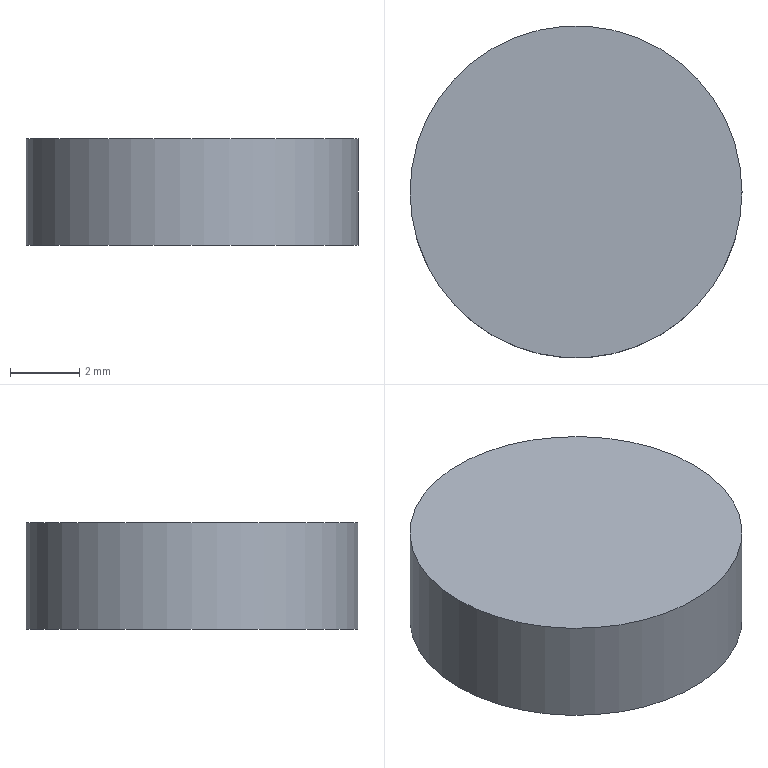Part | STEP file | 1_id338_x_t | 1 solid | 3 faces | box 9.576 x 9.576 x 3.075 mm | volume 221.455 mm3 | plane 2 | cylinder 1 | commonest cylinder face diameters 9.576 x1
STEP:
#1=CARTESIAN_POINT('',(0.,0.,0.));
#2=DIRECTION('',(0.,0.,1.));
#3=DIRECTION('',(1.,0.,0.));
#4=AXIS2_PLACEMENT_3D('',#1,#2,#3);
#5=CARTESIAN_POINT('',(145.212,177.5,-5.));
#6=VERTEX_POINT('',#5);
#7=CARTESIAN_POINT('',(150.,177.5,-5.));
#8=DIRECTION('',(0.,0.,-1.));
#9=DIRECTION('',(-1.,0.,0.));
#10=AXIS2_PLACEMENT_3D('',#7,#8,#9);
#11=CIRCLE('',#10,4.788);
#12=CARTESIAN_POINT('',(150.,177.5,-5.));
#13=DIRECTION('',(0.,0.,-1.));
#14=DIRECTION('',(-1.,0.,0.));
#15=AXIS2_PLACEMENT_3D('',#12,#13,#14);
#16=CYLINDRICAL_SURFACE('',#15,4.788);
#17=CARTESIAN_POINT('',(0.,0.));
#18=DIRECTION('',(1.,0.));
#19=VECTOR('',#18,1.);
#20=LINE('',#17,#19);
#21=(GEOMETRIC_REPRESENTATION_CONTEXT(2)PARAMETRIC_REPRESENTATION_CONTEXT()REPRESENTATION_CONTEXT('',''));
#22=DEFINITIONAL_REPRESENTATION('',(#20),#21);
#23=PCURVE('',#16,#22);
#24=CARTESIAN_POINT('',(150.,177.5,-5.));
#25=DIRECTION('',(0.,0.,-1.));
#26=DIRECTION('',(-1.,0.,0.));
#27=AXIS2_PLACEMENT_3D('',#24,#25,#26);
#28=PLANE('',#27);
#29=CARTESIAN_POINT('',(0.,0.));
#30=DIRECTION('',(1.,0.));
#31=AXIS2_PLACEMENT_2D('',#29,#30);
#32=CIRCLE('',#31,4.788);
#33=(GEOMETRIC_REPRESENTATION_CONTEXT(2)PARAMETRIC_REPRESENTATION_CONTEXT()REPRESENTATION_CONTEXT('',''));
#34=DEFINITIONAL_REPRESENTATION('',(#32),#33);
#35=PCURVE('',#28,#34);
#36=SURFACE_CURVE('',#11,(#23,#35),.PCURVE_S1.);
#37=EDGE_CURVE('',#6,#6,#36,.T.);
#38=ORIENTED_EDGE('',*,*,#37,.T.);
#39=CARTESIAN_POINT('',(145.212,177.5,-8.075));
#40=VERTEX_POINT('',#39);
#41=CARTESIAN_POINT('',(145.212,177.5,-5.));
#42=CARTESIAN_POINT('',(145.212,177.5,-8.075));
#43=B_SPLINE_CURVE_WITH_KNOTS('',1,(#41,#42),.UNSPECIFIED.,.F.,.F.,(2,2),(0.,3.075),.PIECEWISE_BEZIER_KNOTS.);
#44=CARTESIAN_POINT('',(6.283,0.));
#45=DIRECTION('',(0.,1.));
#46=VECTOR('',#45,1.);
#47=LINE('',#44,#46);
#48=(GEOMETRIC_REPRESENTATION_CONTEXT(2)PARAMETRIC_REPRESENTATION_CONTEXT()REPRESENTATION_CONTEXT('',''));
#49=DEFINITIONAL_REPRESENTATION('',(#47),#48);
#50=PCURVE('',#16,#49);
#51=CARTESIAN_POINT('',(0.,0.));
#52=DIRECTION('',(0.,1.));
#53=VECTOR('',#52,1.);
#54=LINE('',#51,#53);
#55=(GEOMETRIC_REPRESENTATION_CONTEXT(2)PARAMETRIC_REPRESENTATION_CONTEXT()REPRESENTATION_CONTEXT('',''));
#56=DEFINITIONAL_REPRESENTATION('',(#54),#55);
#57=PCURVE('',#16,#56);
#58=SEAM_CURVE('',#43,(#50,#57),.PCURVE_S1.);
#59=EDGE_CURVE('',#6,#40,#58,.T.);
#60=ORIENTED_EDGE('',*,*,#59,.T.);
#61=CARTESIAN_POINT('',(150.,177.5,-8.075));
#62=DIRECTION('',(0.,0.,-1.));
#63=DIRECTION('',(-1.,0.,0.));
#64=AXIS2_PLACEMENT_3D('',#61,#62,#63);
#65=CIRCLE('',#64,4.788);
#66=CARTESIAN_POINT('',(0.,3.075));
#67=DIRECTION('',(1.,0.));
#68=VECTOR('',#67,1.);
#69=LINE('',#66,#68);
#70=(GEOMETRIC_REPRESENTATION_CONTEXT(2)PARAMETRIC_REPRESENTATION_CONTEXT()REPRESENTATION_CONTEXT('',''));
#71=DEFINITIONAL_REPRESENTATION('',(#69),#70);
#72=PCURVE('',#16,#71);
#73=CARTESIAN_POINT('',(150.,177.5,-8.075));
#74=DIRECTION('',(0.,0.,-1.));
#75=DIRECTION('',(-1.,0.,0.));
#76=AXIS2_PLACEMENT_3D('',#73,#74,#75);
#77=PLANE('',#76);
#78=CARTESIAN_POINT('',(0.,0.));
#79=DIRECTION('',(1.,0.));
#80=AXIS2_PLACEMENT_2D('',#78,#79);
#81=CIRCLE('',#80,4.788);
#82=(GEOMETRIC_REPRESENTATION_CONTEXT(2)PARAMETRIC_REPRESENTATION_CONTEXT()REPRESENTATION_CONTEXT('',''));
#83=DEFINITIONAL_REPRESENTATION('',(#81),#82);
#84=PCURVE('',#77,#83);
#85=SURFACE_CURVE('',#65,(#72,#84),.PCURVE_S1.);
#86=EDGE_CURVE('',#40,#40,#85,.T.);
#87=ORIENTED_EDGE('',*,*,#86,.F.);
#88=ORIENTED_EDGE('',*,*,#59,.F.);
#89=EDGE_LOOP('',(#38,#60,#87,#88));
#90=FACE_BOUND('',#89,.T.);
#91=ADVANCED_FACE('',(#90),#16,.T.);
#92=ORIENTED_EDGE('',*,*,#37,.F.);
#93=EDGE_LOOP('',(#92));
#94=FACE_BOUND('',#93,.T.);
#95=ADVANCED_FACE('',(#94),#28,.F.);
#96=ORIENTED_EDGE('',*,*,#86,.T.);
#97=EDGE_LOOP('',(#96));
#98=FACE_BOUND('',#97,.T.);
#99=ADVANCED_FACE('',(#98),#77,.T.);
#100=CLOSED_SHELL('',(#91,#95,#99));
#101=MANIFOLD_SOLID_BREP('',#100);
#102=(LENGTH_UNIT()NAMED_UNIT(*)SI_UNIT(.MILLI.,.METRE.));
#103=UNCERTAINTY_MEASURE_WITH_UNIT(LENGTH_MEASURE(0.00001),#102,'','');
#104=(NAMED_UNIT(*)PLANE_ANGLE_UNIT()SI_UNIT($,.RADIAN.));
#105=(NAMED_UNIT(*)SI_UNIT($,.STERADIAN.)SOLID_ANGLE_UNIT());
#106=(GEOMETRIC_REPRESENTATION_CONTEXT(3)GLOBAL_UNCERTAINTY_ASSIGNED_CONTEXT((#103))GLOBAL_UNIT_ASSIGNED_CONTEXT((#102,#104,#105))REPRESENTATION_CONTEXT('',''));
#107=ADVANCED_BREP_SHAPE_REPRESENTATION('',(#4,#101),#106);